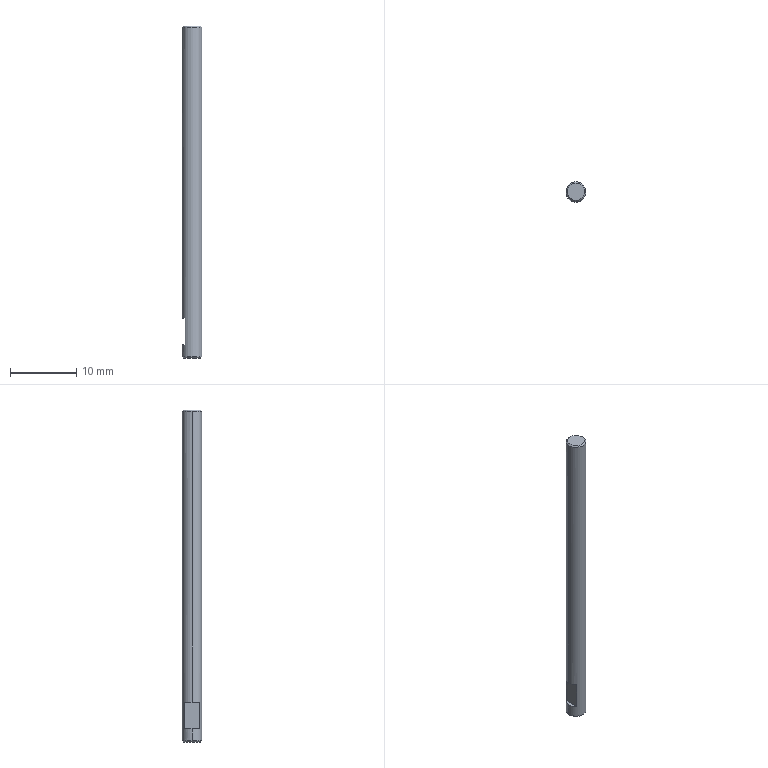Part | SolidWorks | features Chamfer 1, Extrusion 1, ICE 1 | 1 solid | 11 faces | box 3 x 3 x 50 mm | volume 349.971 mm3 | plane 5 | cone 4 | cylinder 2 | commonest cylinder face diameters 3 x2
STEP:
#1=CARTESIAN_POINT('',(-1.3,0.,0.));
#2=VERTEX_POINT('',#1);
#3=CARTESIAN_POINT('',(1.3,0.,0.));
#4=VERTEX_POINT('',#3);
#5=CARTESIAN_POINT('',(0.,0.,0.));
#6=DIRECTION('',(0.,0.,-1.));
#7=DIRECTION('',(1.,0.,0.));
#8=AXIS2_PLACEMENT_3D('',#5,#6,#7);
#9=CIRCLE('',#8,1.3);
#10=EDGE_CURVE('',#2,#4,#9,.T.);
#11=ORIENTED_EDGE('',*,*,#10,.F.);
#12=CARTESIAN_POINT('',(-1.5,0.,0.2));
#13=VERTEX_POINT('',#12);
#14=CARTESIAN_POINT('',(-1.5,0.,0.2));
#15=DIRECTION('',(-0.7071,0.,0.7071));
#16=VECTOR('',#15,1000.);
#17=LINE('',#14,#16);
#18=EDGE_CURVE('',#2,#13,#17,.T.);
#19=ORIENTED_EDGE('',*,*,#18,.T.);
#20=CARTESIAN_POINT('',(1.5,0.,0.2));
#21=VERTEX_POINT('',#20);
#22=CARTESIAN_POINT('',(0.,0.,0.2));
#23=DIRECTION('',(0.,0.,1.));
#24=DIRECTION('',(1.,0.,0.));
#25=AXIS2_PLACEMENT_3D('',#22,#23,#24);
#26=CIRCLE('',#25,1.5);
#27=EDGE_CURVE('',#21,#13,#26,.T.);
#28=ORIENTED_EDGE('',*,*,#27,.F.);
#29=CARTESIAN_POINT('',(1.5,0.,0.2));
#30=DIRECTION('',(0.7071,0.,0.7071));
#31=VECTOR('',#30,1000.);
#32=LINE('',#29,#31);
#33=EDGE_CURVE('',#4,#21,#32,.T.);
#34=ORIENTED_EDGE('',*,*,#33,.F.);
#35=EDGE_LOOP('',(#11,#19,#28,#34));
#36=FACE_OUTER_BOUND('',#35,.T.);
#37=CARTESIAN_POINT('',(0.,0.,0.2));
#38=DIRECTION('',(0.,0.,1.));
#39=DIRECTION('',(1.,0.,0.));
#40=AXIS2_PLACEMENT_3D('',#37,#38,#39);
#41=CONICAL_SURFACE('',#40,1.5,0.7854);
#42=ADVANCED_FACE('',(#36),#41,.T.);
#43=CARTESIAN_POINT('',(1.3,0.,50.));
#44=VERTEX_POINT('',#43);
#45=CARTESIAN_POINT('',(-1.3,0.,50.));
#46=VERTEX_POINT('',#45);
#47=CARTESIAN_POINT('',(0.,0.,50.));
#48=DIRECTION('',(0.,0.,1.));
#49=DIRECTION('',(1.,0.,0.));
#50=AXIS2_PLACEMENT_3D('',#47,#48,#49);
#51=CIRCLE('',#50,1.3);
#52=EDGE_CURVE('',#44,#46,#51,.T.);
#53=ORIENTED_EDGE('',*,*,#52,.F.);
#54=CARTESIAN_POINT('',(1.5,0.,49.8));
#55=VERTEX_POINT('',#54);
#56=CARTESIAN_POINT('',(1.3,0.,50.));
#57=DIRECTION('',(0.7071,0.,-0.7071));
#58=VECTOR('',#57,1000.);
#59=LINE('',#56,#58);
#60=EDGE_CURVE('',#44,#55,#59,.T.);
#61=ORIENTED_EDGE('',*,*,#60,.T.);
#62=CARTESIAN_POINT('',(-1.5,0.,49.8));
#63=VERTEX_POINT('',#62);
#64=CARTESIAN_POINT('',(0.,0.,49.8));
#65=DIRECTION('',(0.,0.,-1.));
#66=DIRECTION('',(1.,0.,0.));
#67=AXIS2_PLACEMENT_3D('',#64,#65,#66);
#68=CIRCLE('',#67,1.5);
#69=EDGE_CURVE('',#63,#55,#68,.T.);
#70=ORIENTED_EDGE('',*,*,#69,.F.);
#71=CARTESIAN_POINT('',(-1.3,0.,50.));
#72=DIRECTION('',(-0.7071,0.,-0.7071));
#73=VECTOR('',#72,1000.);
#74=LINE('',#71,#73);
#75=EDGE_CURVE('',#46,#63,#74,.T.);
#76=ORIENTED_EDGE('',*,*,#75,.F.);
#77=EDGE_LOOP('',(#53,#61,#70,#76));
#78=FACE_OUTER_BOUND('',#77,.T.);
#79=CARTESIAN_POINT('',(0.,0.,50.));
#80=DIRECTION('',(0.,0.,-1.));
#81=DIRECTION('',(-1.,0.,0.));
#82=AXIS2_PLACEMENT_3D('',#79,#80,#81);
#83=CONICAL_SURFACE('',#82,1.3,0.7854);
#84=ADVANCED_FACE('',(#78),#83,.T.);
#85=ORIENTED_EDGE('',*,*,#69,.T.);
#86=CARTESIAN_POINT('',(1.5,0.,50.));
#87=DIRECTION('',(0.,0.,-1.));
#88=VECTOR('',#87,1000.);
#89=LINE('',#86,#88);
#90=EDGE_CURVE('',#55,#21,#89,.T.);
#91=ORIENTED_EDGE('',*,*,#90,.T.);
#92=ORIENTED_EDGE('',*,*,#27,.T.);
#93=CARTESIAN_POINT('',(-1.5,0.,2.));
#94=VERTEX_POINT('',#93);
#95=CARTESIAN_POINT('',(-1.5,0.,50.));
#96=DIRECTION('',(0.,0.,-1.));
#97=VECTOR('',#96,1000.);
#98=LINE('',#95,#97);
#99=EDGE_CURVE('',#94,#13,#98,.T.);
#100=ORIENTED_EDGE('',*,*,#99,.F.);
#101=CARTESIAN_POINT('',(-1.,1.118,2.));
#102=VERTEX_POINT('',#101);
#103=CARTESIAN_POINT('',(0.,0.,2.));
#104=DIRECTION('',(0.,0.,-1.));
#105=DIRECTION('',(-1.,0.,0.));
#106=AXIS2_PLACEMENT_3D('',#103,#104,#105);
#107=CIRCLE('',#106,1.5);
#108=EDGE_CURVE('',#94,#102,#107,.T.);
#109=ORIENTED_EDGE('',*,*,#108,.T.);
#110=CARTESIAN_POINT('',(-1.,1.118,6.));
#111=VERTEX_POINT('',#110);
#112=CARTESIAN_POINT('',(-1.,1.118,50.));
#113=DIRECTION('',(0.,0.,1.));
#114=VECTOR('',#113,1000.);
#115=LINE('',#112,#114);
#116=EDGE_CURVE('',#102,#111,#115,.T.);
#117=ORIENTED_EDGE('',*,*,#116,.T.);
#118=CARTESIAN_POINT('',(-1.5,0.,6.));
#119=VERTEX_POINT('',#118);
#120=CARTESIAN_POINT('',(0.,0.,6.));
#121=DIRECTION('',(0.,0.,1.));
#122=DIRECTION('',(1.,0.,0.));
#123=AXIS2_PLACEMENT_3D('',#120,#121,#122);
#124=CIRCLE('',#123,1.5);
#125=EDGE_CURVE('',#111,#119,#124,.T.);
#126=ORIENTED_EDGE('',*,*,#125,.T.);
#127=CARTESIAN_POINT('',(-1.5,0.,50.));
#128=DIRECTION('',(0.,0.,-1.));
#129=VECTOR('',#128,1000.);
#130=LINE('',#127,#129);
#131=EDGE_CURVE('',#63,#119,#130,.T.);
#132=ORIENTED_EDGE('',*,*,#131,.F.);
#133=EDGE_LOOP('',(#85,#91,#92,#100,#109,#117,#126,#132));
#134=FACE_OUTER_BOUND('',#133,.T.);
#135=CARTESIAN_POINT('',(0.,0.,50.));
#136=DIRECTION('',(0.,0.,-1.));
#137=DIRECTION('',(-1.,0.,0.));
#138=AXIS2_PLACEMENT_3D('',#135,#136,#137);
#139=CYLINDRICAL_SURFACE('',#138,1.5);
#140=ADVANCED_FACE('',(#134),#139,.T.);
#141=ORIENTED_EDGE('',*,*,#90,.F.);
#142=CARTESIAN_POINT('',(0.,0.,49.8));
#143=DIRECTION('',(0.,0.,-1.));
#144=DIRECTION('',(1.,0.,0.));
#145=AXIS2_PLACEMENT_3D('',#142,#143,#144);
#146=CIRCLE('',#145,1.5);
#147=EDGE_CURVE('',#55,#63,#146,.T.);
#148=ORIENTED_EDGE('',*,*,#147,.T.);
#149=ORIENTED_EDGE('',*,*,#131,.T.);
#150=CARTESIAN_POINT('',(-1.,-1.118,6.));
#151=VERTEX_POINT('',#150);
#152=CARTESIAN_POINT('',(0.,0.,6.));
#153=DIRECTION('',(0.,0.,1.));
#154=DIRECTION('',(1.,0.,0.));
#155=AXIS2_PLACEMENT_3D('',#152,#153,#154);
#156=CIRCLE('',#155,1.5);
#157=EDGE_CURVE('',#119,#151,#156,.T.);
#158=ORIENTED_EDGE('',*,*,#157,.T.);
#159=CARTESIAN_POINT('',(-1.,-1.118,2.));
#160=VERTEX_POINT('',#159);
#161=CARTESIAN_POINT('',(-1.,-1.118,50.));
#162=DIRECTION('',(0.,0.,-1.));
#163=VECTOR('',#162,1000.);
#164=LINE('',#161,#163);
#165=EDGE_CURVE('',#151,#160,#164,.T.);
#166=ORIENTED_EDGE('',*,*,#165,.T.);
#167=CARTESIAN_POINT('',(0.,0.,2.));
#168=DIRECTION('',(0.,0.,-1.));
#169=DIRECTION('',(-1.,0.,0.));
#170=AXIS2_PLACEMENT_3D('',#167,#168,#169);
#171=CIRCLE('',#170,1.5);
#172=EDGE_CURVE('',#160,#94,#171,.T.);
#173=ORIENTED_EDGE('',*,*,#172,.T.);
#174=ORIENTED_EDGE('',*,*,#99,.T.);
#175=CARTESIAN_POINT('',(0.,0.,0.2));
#176=DIRECTION('',(0.,0.,1.));
#177=DIRECTION('',(1.,0.,0.));
#178=AXIS2_PLACEMENT_3D('',#175,#176,#177);
#179=CIRCLE('',#178,1.5);
#180=EDGE_CURVE('',#13,#21,#179,.T.);
#181=ORIENTED_EDGE('',*,*,#180,.T.);
#182=EDGE_LOOP('',(#141,#148,#149,#158,#166,#173,#174,#181));
#183=FACE_OUTER_BOUND('',#182,.T.);
#184=CARTESIAN_POINT('',(0.,0.,50.));
#185=DIRECTION('',(0.,0.,-1.));
#186=DIRECTION('',(-1.,0.,0.));
#187=AXIS2_PLACEMENT_3D('',#184,#185,#186);
#188=CYLINDRICAL_SURFACE('',#187,1.5);
#189=ADVANCED_FACE('',(#183),#188,.T.);
#190=CARTESIAN_POINT('',(0.,0.,50.));
#191=DIRECTION('',(0.,0.,1.));
#192=DIRECTION('',(1.,0.,0.));
#193=AXIS2_PLACEMENT_3D('',#190,#191,#192);
#194=CIRCLE('',#193,1.3);
#195=EDGE_CURVE('',#46,#44,#194,.T.);
#196=ORIENTED_EDGE('',*,*,#195,.T.);
#197=ORIENTED_EDGE('',*,*,#52,.T.);
#198=EDGE_LOOP('',(#196,#197));
#199=FACE_OUTER_BOUND('',#198,.T.);
#200=CARTESIAN_POINT('',(0.,0.,50.));
#201=DIRECTION('',(0.,0.,1.));
#202=DIRECTION('',(1.,0.,0.));
#203=AXIS2_PLACEMENT_3D('',#200,#201,#202);
#204=PLANE('',#203);
#205=ADVANCED_FACE('',(#199),#204,.T.);
#206=CARTESIAN_POINT('',(0.,0.,0.));
#207=DIRECTION('',(0.,0.,-1.));
#208=DIRECTION('',(1.,0.,0.));
#209=AXIS2_PLACEMENT_3D('',#206,#207,#208);
#210=CIRCLE('',#209,1.3);
#211=EDGE_CURVE('',#4,#2,#210,.T.);
#212=ORIENTED_EDGE('',*,*,#211,.T.);
#213=ORIENTED_EDGE('',*,*,#10,.T.);
#214=EDGE_LOOP('',(#212,#213));
#215=FACE_OUTER_BOUND('',#214,.T.);
#216=CARTESIAN_POINT('',(0.,0.,0.));
#217=DIRECTION('',(0.,0.,1.));
#218=DIRECTION('',(1.,0.,0.));
#219=AXIS2_PLACEMENT_3D('',#216,#217,#218);
#220=PLANE('',#219);
#221=ADVANCED_FACE('',(#215),#220,.F.);
#222=ORIENTED_EDGE('',*,*,#172,.F.);
#223=CARTESIAN_POINT('',(-1.,-15.,2.));
#224=DIRECTION('',(0.,1.,0.));
#225=VECTOR('',#224,1000.);
#226=LINE('',#223,#225);
#227=EDGE_CURVE('',#160,#102,#226,.T.);
#228=ORIENTED_EDGE('',*,*,#227,.T.);
#229=ORIENTED_EDGE('',*,*,#108,.F.);
#230=EDGE_LOOP('',(#222,#228,#229));
#231=FACE_OUTER_BOUND('',#230,.T.);
#232=CARTESIAN_POINT('',(-1.5,-15.,2.));
#233=DIRECTION('',(0.,0.,-1.));
#234=DIRECTION('',(-1.,0.,0.));
#235=AXIS2_PLACEMENT_3D('',#232,#233,#234);
#236=PLANE('',#235);
#237=ADVANCED_FACE('',(#231),#236,.F.);
#238=CARTESIAN_POINT('',(-1.,-15.,6.));
#239=DIRECTION('',(0.,1.,0.));
#240=VECTOR('',#239,1000.);
#241=LINE('',#238,#240);
#242=EDGE_CURVE('',#151,#111,#241,.T.);
#243=ORIENTED_EDGE('',*,*,#242,.T.);
#244=ORIENTED_EDGE('',*,*,#116,.F.);
#245=ORIENTED_EDGE('',*,*,#227,.F.);
#246=ORIENTED_EDGE('',*,*,#165,.F.);
#247=EDGE_LOOP('',(#243,#244,#245,#246));
#248=FACE_OUTER_BOUND('',#247,.T.);
#249=CARTESIAN_POINT('',(-1.,-15.,2.));
#250=DIRECTION('',(1.,0.,0.));
#251=DIRECTION('',(0.,0.,-1.));
#252=AXIS2_PLACEMENT_3D('',#249,#250,#251);
#253=PLANE('',#252);
#254=ADVANCED_FACE('',(#248),#253,.F.);
#255=ORIENTED_EDGE('',*,*,#242,.F.);
#256=ORIENTED_EDGE('',*,*,#157,.F.);
#257=ORIENTED_EDGE('',*,*,#125,.F.);
#258=EDGE_LOOP('',(#255,#256,#257));
#259=FACE_OUTER_BOUND('',#258,.T.);
#260=CARTESIAN_POINT('',(-1.5,-15.,6.));
#261=DIRECTION('',(0.,0.,1.));
#262=DIRECTION('',(1.,0.,0.));
#263=AXIS2_PLACEMENT_3D('',#260,#261,#262);
#264=PLANE('',#263);
#265=ADVANCED_FACE('',(#259),#264,.F.);
#266=ORIENTED_EDGE('',*,*,#60,.F.);
#267=ORIENTED_EDGE('',*,*,#195,.F.);
#268=ORIENTED_EDGE('',*,*,#75,.T.);
#269=ORIENTED_EDGE('',*,*,#147,.F.);
#270=EDGE_LOOP('',(#266,#267,#268,#269));
#271=FACE_OUTER_BOUND('',#270,.T.);
#272=CARTESIAN_POINT('',(0.,0.,50.));
#273=DIRECTION('',(0.,0.,-1.));
#274=DIRECTION('',(-1.,0.,0.));
#275=AXIS2_PLACEMENT_3D('',#272,#273,#274);
#276=CONICAL_SURFACE('',#275,1.3,0.7854);
#277=ADVANCED_FACE('',(#271),#276,.T.);
#278=ORIENTED_EDGE('',*,*,#18,.F.);
#279=ORIENTED_EDGE('',*,*,#211,.F.);
#280=ORIENTED_EDGE('',*,*,#33,.T.);
#281=ORIENTED_EDGE('',*,*,#180,.F.);
#282=EDGE_LOOP('',(#278,#279,#280,#281));
#283=FACE_OUTER_BOUND('',#282,.T.);
#284=CARTESIAN_POINT('',(0.,0.,0.2));
#285=DIRECTION('',(0.,0.,1.));
#286=DIRECTION('',(1.,0.,0.));
#287=AXIS2_PLACEMENT_3D('',#284,#285,#286);
#288=CONICAL_SURFACE('',#287,1.5,0.7854);
#289=ADVANCED_FACE('',(#283),#288,.T.);
#290=CLOSED_SHELL('',(#42,#84,#140,#189,#205,#221,#237,#254,#265,#277,#289));
#291=MANIFOLD_SOLID_BREP('',#290);
#292=CARTESIAN_POINT('',(0.,0.,0.));
#293=DIRECTION('',(0.,0.,1.));
#294=DIRECTION('',(1.,0.,0.));
#295=AXIS2_PLACEMENT_3D('',#292,#293,#294);
#296=(LENGTH_UNIT()NAMED_UNIT(*)SI_UNIT(.MILLI.,.METRE.));
#297=UNCERTAINTY_MEASURE_WITH_UNIT(LENGTH_MEASURE(0.00001),#296,'','');
#298=(NAMED_UNIT(*)PLANE_ANGLE_UNIT()SI_UNIT($,.RADIAN.));
#299=(NAMED_UNIT(*)SI_UNIT($,.STERADIAN.)SOLID_ANGLE_UNIT());
#300=(GEOMETRIC_REPRESENTATION_CONTEXT(3)GLOBAL_UNCERTAINTY_ASSIGNED_CONTEXT((#297))GLOBAL_UNIT_ASSIGNED_CONTEXT((#296,#298,#299))REPRESENTATION_CONTEXT('',''));
#301=ADVANCED_BREP_SHAPE_REPRESENTATION('',(#291,#295),#300);